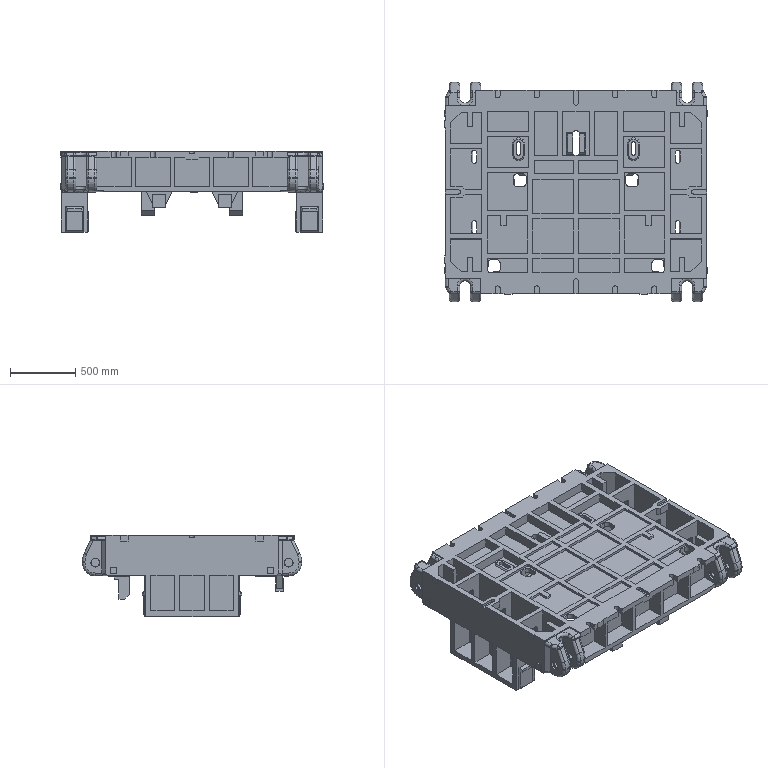Part | NX | features solid 2 | 1 solid | 1449 faces | box 2020 x 1680 x 625 mm | volume 373094517 mm3 | plane 1093 | cylinder 266 | torus 40 | cone 34 | sphere 16 | commonest cylinder face diameters 40 x128 68 x48 60 x16 64 x16 20 x12 80 x10